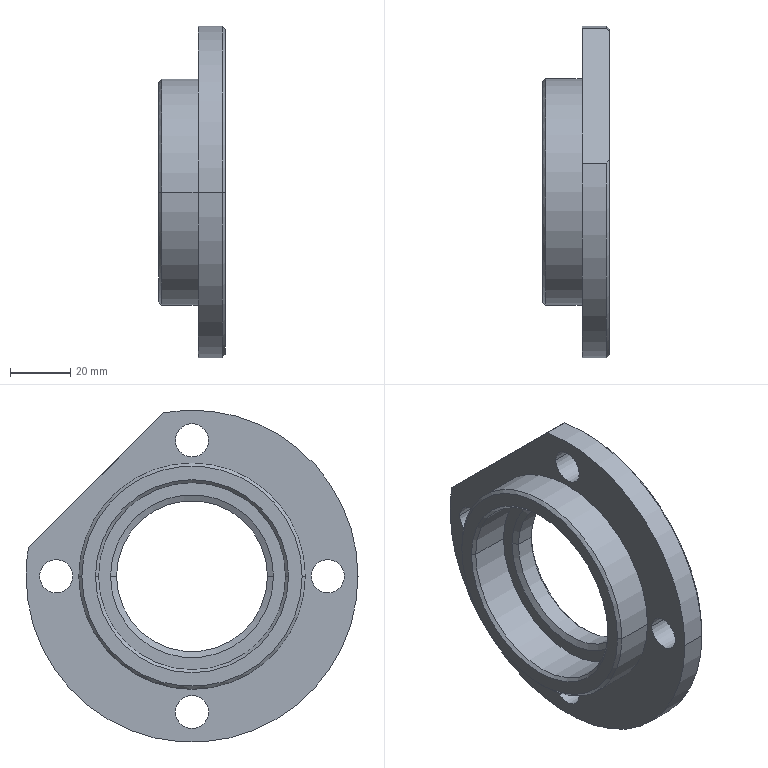Part | SolidWorks | features BaseBody 1 | 1 solid | 33 faces | box 22 x 110 x 110 mm | volume 77102 mm3 | cylinder 17 | cone 11 | plane 5 | commonest cylinder face diameters 11 x8 110 x3 50 x2 62 x2 75 x2
STEP:
#1=CARTESIAN_POINT('',(8.,-25.,0.));
#2=VERTEX_POINT('',#1);
#3=CARTESIAN_POINT('',(8.,25.,0.));
#4=VERTEX_POINT('',#3);
#5=CARTESIAN_POINT('',(8.,0.,0.));
#6=DIRECTION('',(1.,0.,0.));
#7=DIRECTION('',(0.,-1.,0.));
#8=AXIS2_PLACEMENT_3D('',#5,#6,#7);
#9=CIRCLE('',#8,25.);
#10=EDGE_CURVE('',#2,#4,#9,.T.);
#11=ORIENTED_EDGE('',*,*,#10,.F.);
#12=CARTESIAN_POINT('',(9.,-26.,0.));
#13=VERTEX_POINT('',#12);
#14=CARTESIAN_POINT('',(9.,-26.,0.));
#15=DIRECTION('',(0.7071,-0.7071,0.));
#16=VECTOR('',#15,1000.);
#17=LINE('',#14,#16);
#18=EDGE_CURVE('',#2,#13,#17,.T.);
#19=ORIENTED_EDGE('',*,*,#18,.T.);
#20=CARTESIAN_POINT('',(9.,26.,0.));
#21=VERTEX_POINT('',#20);
#22=CARTESIAN_POINT('',(9.,0.,0.));
#23=DIRECTION('',(-1.,0.,0.));
#24=DIRECTION('',(0.,1.,0.));
#25=AXIS2_PLACEMENT_3D('',#22,#23,#24);
#26=CIRCLE('',#25,26.);
#27=EDGE_CURVE('',#21,#13,#26,.T.);
#28=ORIENTED_EDGE('',*,*,#27,.F.);
#29=CARTESIAN_POINT('',(9.,26.,0.));
#30=DIRECTION('',(0.7071,0.7071,0.));
#31=VECTOR('',#30,1000.);
#32=LINE('',#29,#31);
#33=EDGE_CURVE('',#4,#21,#32,.T.);
#34=ORIENTED_EDGE('',*,*,#33,.F.);
#35=EDGE_LOOP('',(#11,#19,#28,#34));
#36=FACE_OUTER_BOUND('',#35,.T.);
#37=CARTESIAN_POINT('',(9.,0.,0.));
#38=DIRECTION('',(1.,0.,0.));
#39=DIRECTION('',(0.,1.,0.));
#40=AXIS2_PLACEMENT_3D('',#37,#38,#39);
#41=CONICAL_SURFACE('',#40,26.,0.7854);
#42=ADVANCED_FACE('',(#36),#41,.F.);
#43=CARTESIAN_POINT('',(0.,39.5,0.));
#44=VERTEX_POINT('',#43);
#45=CARTESIAN_POINT('',(0.,50.5,0.));
#46=VERTEX_POINT('',#45);
#47=CARTESIAN_POINT('',(0.,45.,0.));
#48=DIRECTION('',(1.,0.,0.));
#49=DIRECTION('',(0.,1.,0.));
#50=AXIS2_PLACEMENT_3D('',#47,#48,#49);
#51=CIRCLE('',#50,5.5);
#52=EDGE_CURVE('',#44,#46,#51,.T.);
#53=ORIENTED_EDGE('',*,*,#52,.F.);
#54=CARTESIAN_POINT('',(9.,39.5,0.));
#55=VERTEX_POINT('',#54);
#56=CARTESIAN_POINT('',(-148.111,39.5,0.));
#57=DIRECTION('',(1.,0.,0.));
#58=VECTOR('',#57,1000.);
#59=LINE('',#56,#58);
#60=EDGE_CURVE('',#44,#55,#59,.T.);
#61=ORIENTED_EDGE('',*,*,#60,.T.);
#62=CARTESIAN_POINT('',(9.,50.5,0.));
#63=VERTEX_POINT('',#62);
#64=CARTESIAN_POINT('',(9.,45.,0.));
#65=DIRECTION('',(-1.,0.,0.));
#66=DIRECTION('',(0.,1.,0.));
#67=AXIS2_PLACEMENT_3D('',#64,#65,#66);
#68=CIRCLE('',#67,5.5);
#69=EDGE_CURVE('',#63,#55,#68,.T.);
#70=ORIENTED_EDGE('',*,*,#69,.F.);
#71=CARTESIAN_POINT('',(-148.111,50.5,0.));
#72=DIRECTION('',(1.,0.,0.));
#73=VECTOR('',#72,1000.);
#74=LINE('',#71,#73);
#75=EDGE_CURVE('',#46,#63,#74,.T.);
#76=ORIENTED_EDGE('',*,*,#75,.F.);
#77=EDGE_LOOP('',(#53,#61,#70,#76));
#78=FACE_OUTER_BOUND('',#77,.T.);
#79=CARTESIAN_POINT('',(-148.111,45.,0.));
#80=DIRECTION('',(1.,0.,0.));
#81=DIRECTION('',(0.,1.,0.));
#82=AXIS2_PLACEMENT_3D('',#79,#80,#81);
#83=CYLINDRICAL_SURFACE('',#82,5.5);
#84=ADVANCED_FACE('',(#78),#83,.F.);
#85=CARTESIAN_POINT('',(0.,-5.5,45.));
#86=VERTEX_POINT('',#85);
#87=CARTESIAN_POINT('',(0.,5.5,45.));
#88=VERTEX_POINT('',#87);
#89=CARTESIAN_POINT('',(0.,0.,45.));
#90=DIRECTION('',(1.,0.,0.));
#91=DIRECTION('',(0.,1.,0.));
#92=AXIS2_PLACEMENT_3D('',#89,#90,#91);
#93=CIRCLE('',#92,5.5);
#94=EDGE_CURVE('',#86,#88,#93,.T.);
#95=ORIENTED_EDGE('',*,*,#94,.F.);
#96=CARTESIAN_POINT('',(9.,-5.5,45.));
#97=VERTEX_POINT('',#96);
#98=CARTESIAN_POINT('',(-148.111,-5.5,45.));
#99=DIRECTION('',(1.,0.,0.));
#100=VECTOR('',#99,1000.);
#101=LINE('',#98,#100);
#102=EDGE_CURVE('',#86,#97,#101,.T.);
#103=ORIENTED_EDGE('',*,*,#102,.T.);
#104=CARTESIAN_POINT('',(9.,5.5,45.));
#105=VERTEX_POINT('',#104);
#106=CARTESIAN_POINT('',(9.,0.,45.));
#107=DIRECTION('',(-1.,0.,0.));
#108=DIRECTION('',(0.,1.,0.));
#109=AXIS2_PLACEMENT_3D('',#106,#107,#108);
#110=CIRCLE('',#109,5.5);
#111=EDGE_CURVE('',#105,#97,#110,.T.);
#112=ORIENTED_EDGE('',*,*,#111,.F.);
#113=CARTESIAN_POINT('',(-148.111,5.5,45.));
#114=DIRECTION('',(1.,0.,0.));
#115=VECTOR('',#114,1000.);
#116=LINE('',#113,#115);
#117=EDGE_CURVE('',#88,#105,#116,.T.);
#118=ORIENTED_EDGE('',*,*,#117,.F.);
#119=EDGE_LOOP('',(#95,#103,#112,#118));
#120=FACE_OUTER_BOUND('',#119,.T.);
#121=CARTESIAN_POINT('',(-148.111,0.,45.));
#122=DIRECTION('',(1.,0.,0.));
#123=DIRECTION('',(0.,1.,0.));
#124=AXIS2_PLACEMENT_3D('',#121,#122,#123);
#125=CYLINDRICAL_SURFACE('',#124,5.5);
#126=ADVANCED_FACE('',(#120),#125,.F.);
#127=CARTESIAN_POINT('',(0.,-50.5,0.));
#128=VERTEX_POINT('',#127);
#129=CARTESIAN_POINT('',(0.,-39.5,0.));
#130=VERTEX_POINT('',#129);
#131=CARTESIAN_POINT('',(0.,-45.,0.));
#132=DIRECTION('',(1.,0.,0.));
#133=DIRECTION('',(0.,1.,0.));
#134=AXIS2_PLACEMENT_3D('',#131,#132,#133);
#135=CIRCLE('',#134,5.5);
#136=EDGE_CURVE('',#128,#130,#135,.T.);
#137=ORIENTED_EDGE('',*,*,#136,.F.);
#138=CARTESIAN_POINT('',(9.,-50.5,0.));
#139=VERTEX_POINT('',#138);
#140=CARTESIAN_POINT('',(-148.111,-50.5,0.));
#141=DIRECTION('',(1.,0.,0.));
#142=VECTOR('',#141,1000.);
#143=LINE('',#140,#142);
#144=EDGE_CURVE('',#128,#139,#143,.T.);
#145=ORIENTED_EDGE('',*,*,#144,.T.);
#146=CARTESIAN_POINT('',(9.,-39.5,0.));
#147=VERTEX_POINT('',#146);
#148=CARTESIAN_POINT('',(9.,-45.,0.));
#149=DIRECTION('',(-1.,0.,0.));
#150=DIRECTION('',(0.,1.,0.));
#151=AXIS2_PLACEMENT_3D('',#148,#149,#150);
#152=CIRCLE('',#151,5.5);
#153=EDGE_CURVE('',#147,#139,#152,.T.);
#154=ORIENTED_EDGE('',*,*,#153,.F.);
#155=CARTESIAN_POINT('',(-148.111,-39.5,0.));
#156=DIRECTION('',(1.,0.,0.));
#157=VECTOR('',#156,1000.);
#158=LINE('',#155,#157);
#159=EDGE_CURVE('',#130,#147,#158,.T.);
#160=ORIENTED_EDGE('',*,*,#159,.F.);
#161=EDGE_LOOP('',(#137,#145,#154,#160));
#162=FACE_OUTER_BOUND('',#161,.T.);
#163=CARTESIAN_POINT('',(-148.111,-45.,0.));
#164=DIRECTION('',(1.,0.,0.));
#165=DIRECTION('',(0.,1.,0.));
#166=AXIS2_PLACEMENT_3D('',#163,#164,#165);
#167=CYLINDRICAL_SURFACE('',#166,5.5);
#168=ADVANCED_FACE('',(#162),#167,.F.);
#169=CARTESIAN_POINT('',(0.,-5.5,-45.));
#170=VERTEX_POINT('',#169);
#171=CARTESIAN_POINT('',(0.,5.5,-45.));
#172=VERTEX_POINT('',#171);
#173=CARTESIAN_POINT('',(0.,0.,-45.));
#174=DIRECTION('',(1.,0.,0.));
#175=DIRECTION('',(0.,1.,0.));
#176=AXIS2_PLACEMENT_3D('',#173,#174,#175);
#177=CIRCLE('',#176,5.5);
#178=EDGE_CURVE('',#170,#172,#177,.T.);
#179=ORIENTED_EDGE('',*,*,#178,.F.);
#180=CARTESIAN_POINT('',(9.,-5.5,-45.));
#181=VERTEX_POINT('',#180);
#182=CARTESIAN_POINT('',(-148.111,-5.5,-45.));
#183=DIRECTION('',(1.,0.,0.));
#184=VECTOR('',#183,1000.);
#185=LINE('',#182,#184);
#186=EDGE_CURVE('',#170,#181,#185,.T.);
#187=ORIENTED_EDGE('',*,*,#186,.T.);
#188=CARTESIAN_POINT('',(9.,5.5,-45.));
#189=VERTEX_POINT('',#188);
#190=CARTESIAN_POINT('',(9.,0.,-45.));
#191=DIRECTION('',(-1.,0.,0.));
#192=DIRECTION('',(0.,1.,0.));
#193=AXIS2_PLACEMENT_3D('',#190,#191,#192);
#194=CIRCLE('',#193,5.5);
#195=EDGE_CURVE('',#189,#181,#194,.T.);
#196=ORIENTED_EDGE('',*,*,#195,.F.);
#197=CARTESIAN_POINT('',(-148.111,5.5,-45.));
#198=DIRECTION('',(1.,0.,0.));
#199=VECTOR('',#198,1000.);
#200=LINE('',#197,#199);
#201=EDGE_CURVE('',#172,#189,#200,.T.);
#202=ORIENTED_EDGE('',*,*,#201,.F.);
#203=EDGE_LOOP('',(#179,#187,#196,#202));
#204=FACE_OUTER_BOUND('',#203,.T.);
#205=CARTESIAN_POINT('',(-148.111,0.,-45.));
#206=DIRECTION('',(1.,0.,0.));
#207=DIRECTION('',(0.,1.,0.));
#208=AXIS2_PLACEMENT_3D('',#205,#206,#207);
#209=CYLINDRICAL_SURFACE('',#208,5.5);
#210=ADVANCED_FACE('',(#204),#209,.F.);
#211=CARTESIAN_POINT('',(9.,54.,0.));
#212=VERTEX_POINT('',#211);
#213=CARTESIAN_POINT('',(9.,52.927,10.713));
#214=VERTEX_POINT('',#213);
#215=CARTESIAN_POINT('',(9.,0.,0.));
#216=DIRECTION('',(1.,0.,0.));
#217=DIRECTION('',(0.,-1.,0.));
#218=AXIS2_PLACEMENT_3D('',#215,#216,#217);
#219=CIRCLE('',#218,54.);
#220=EDGE_CURVE('',#212,#214,#219,.T.);
#221=ORIENTED_EDGE('',*,*,#220,.F.);
#222=CARTESIAN_POINT('',(8.,55.,0.));
#223=VERTEX_POINT('',#222);
#224=CARTESIAN_POINT('',(8.,55.,0.));
#225=DIRECTION('',(-0.7071,0.7071,0.));
#226=VECTOR('',#225,1000.);
#227=LINE('',#224,#226);
#228=EDGE_CURVE('',#212,#223,#227,.T.);
#229=ORIENTED_EDGE('',*,*,#228,.T.);
#230=CARTESIAN_POINT('',(8.,54.18,9.459));
#231=VERTEX_POINT('',#230);
#232=CARTESIAN_POINT('',(8.,0.,0.));
#233=DIRECTION('',(1.,0.,0.));
#234=DIRECTION('',(0.,-1.,0.));
#235=AXIS2_PLACEMENT_3D('',#232,#233,#234);
#236=CIRCLE('',#235,55.);
#237=EDGE_CURVE('',#223,#231,#236,.T.);
#238=ORIENTED_EDGE('',*,*,#237,.T.);
#239=CARTESIAN_POINT('',(8.,54.18,9.459));
#240=CARTESIAN_POINT('',(8.338,53.765,9.875));
#241=CARTESIAN_POINT('',(8.672,53.347,10.293));
#242=CARTESIAN_POINT('',(9.,52.927,10.713));
#243=B_SPLINE_CURVE_WITH_KNOTS('',3,(#239,#240,#241,#242),.UNSPECIFIED.,.F.,.F.,(4,4),(0.,0.002036),.UNSPECIFIED.);
#244=EDGE_CURVE('',#231,#214,#243,.T.);
#245=ORIENTED_EDGE('',*,*,#244,.T.);
#246=EDGE_LOOP('',(#221,#229,#238,#245));
#247=FACE_OUTER_BOUND('',#246,.T.);
#248=CARTESIAN_POINT('',(8.,0.,0.));
#249=DIRECTION('',(-1.,0.,0.));
#250=DIRECTION('',(0.,-1.,0.));
#251=AXIS2_PLACEMENT_3D('',#248,#249,#250);
#252=CONICAL_SURFACE('',#251,55.,0.7854);
#253=ADVANCED_FACE('',(#247),#252,.T.);
#254=ORIENTED_EDGE('',*,*,#228,.F.);
#255=CARTESIAN_POINT('',(9.,-54.,0.));
#256=VERTEX_POINT('',#255);
#257=CARTESIAN_POINT('',(9.,0.,0.));
#258=DIRECTION('',(1.,0.,0.));
#259=DIRECTION('',(0.,-1.,0.));
#260=AXIS2_PLACEMENT_3D('',#257,#258,#259);
#261=CIRCLE('',#260,54.);
#262=EDGE_CURVE('',#256,#212,#261,.T.);
#263=ORIENTED_EDGE('',*,*,#262,.F.);
#264=CARTESIAN_POINT('',(8.,-55.,0.));
#265=VERTEX_POINT('',#264);
#266=CARTESIAN_POINT('',(8.,-55.,0.));
#267=DIRECTION('',(-0.7071,-0.7071,0.));
#268=VECTOR('',#267,1000.);
#269=LINE('',#266,#268);
#270=EDGE_CURVE('',#256,#265,#269,.T.);
#271=ORIENTED_EDGE('',*,*,#270,.T.);
#272=CARTESIAN_POINT('',(8.,0.,0.));
#273=DIRECTION('',(1.,0.,0.));
#274=DIRECTION('',(0.,-1.,0.));
#275=AXIS2_PLACEMENT_3D('',#272,#273,#274);
#276=CIRCLE('',#275,55.);
#277=EDGE_CURVE('',#265,#223,#276,.T.);
#278=ORIENTED_EDGE('',*,*,#277,.T.);
#279=EDGE_LOOP('',(#254,#263,#271,#278));
#280=FACE_OUTER_BOUND('',#279,.T.);
#281=CARTESIAN_POINT('',(8.,0.,0.));
#282=DIRECTION('',(-1.,0.,0.));
#283=DIRECTION('',(0.,-1.,0.));
#284=AXIS2_PLACEMENT_3D('',#281,#282,#283);
#285=CONICAL_SURFACE('',#284,55.,0.7854);
#286=ADVANCED_FACE('',(#280),#285,.T.);
#287=CARTESIAN_POINT('',(2.,-25.,0.));
#288=VERTEX_POINT('',#287);
#289=CARTESIAN_POINT('',(2.,25.,0.));
#290=VERTEX_POINT('',#289);
#291=CARTESIAN_POINT('',(2.,0.,0.));
#292=DIRECTION('',(1.,0.,0.));
#293=DIRECTION('',(0.,1.,0.));
#294=AXIS2_PLACEMENT_3D('',#291,#292,#293);
#295=CIRCLE('',#294,25.);
#296=EDGE_CURVE('',#288,#290,#295,.T.);
#297=ORIENTED_EDGE('',*,*,#296,.F.);
#298=CARTESIAN_POINT('',(5.,-25.,0.));
#299=DIRECTION('',(1.,0.,0.));
#300=VECTOR('',#299,1000.);
#301=LINE('',#298,#300);
#302=EDGE_CURVE('',#288,#2,#301,.T.);
#303=ORIENTED_EDGE('',*,*,#302,.T.);
#304=ORIENTED_EDGE('',*,*,#10,.T.);
#305=CARTESIAN_POINT('',(5.,25.,0.));
#306=DIRECTION('',(1.,0.,0.));
#307=VECTOR('',#306,1000.);
#308=LINE('',#305,#307);
#309=EDGE_CURVE('',#290,#4,#308,.T.);
#310=ORIENTED_EDGE('',*,*,#309,.F.);
#311=EDGE_LOOP('',(#297,#303,#304,#310));
#312=FACE_OUTER_BOUND('',#311,.T.);
#313=CARTESIAN_POINT('',(5.,0.,0.));
#314=DIRECTION('',(1.,0.,0.));
#315=DIRECTION('',(0.,1.,0.));
#316=AXIS2_PLACEMENT_3D('',#313,#314,#315);
#317=CYLINDRICAL_SURFACE('',#316,25.);
#318=ADVANCED_FACE('',(#312),#317,.F.);
#319=CARTESIAN_POINT('',(0.,-55.,0.));
#320=VERTEX_POINT('',#319);
#321=CARTESIAN_POINT('',(0.,9.459,54.18));
#322=VERTEX_POINT('',#321);
#323=CARTESIAN_POINT('',(0.,0.,0.));
#324=DIRECTION('',(-1.,0.,0.));
#325=DIRECTION('',(0.,1.,0.));
#326=AXIS2_PLACEMENT_3D('',#323,#324,#325);
#327=CIRCLE('',#326,55.);
#328=EDGE_CURVE('',#320,#322,#327,.T.);
#329=ORIENTED_EDGE('',*,*,#328,.F.);
#330=CARTESIAN_POINT('',(4.5,-55.,0.));
#331=DIRECTION('',(1.,0.,0.));
#332=VECTOR('',#331,1000.);
#333=LINE('',#330,#332);
#334=EDGE_CURVE('',#320,#265,#333,.T.);
#335=ORIENTED_EDGE('',*,*,#334,.T.);
#336=CARTESIAN_POINT('',(8.,9.459,54.18));
#337=VERTEX_POINT('',#336);
#338=CARTESIAN_POINT('',(8.,0.,0.));
#339=DIRECTION('',(1.,0.,0.));
#340=DIRECTION('',(0.,-1.,0.));
#341=AXIS2_PLACEMENT_3D('',#338,#339,#340);
#342=CIRCLE('',#341,55.);
#343=EDGE_CURVE('',#337,#265,#342,.T.);
#344=ORIENTED_EDGE('',*,*,#343,.F.);
#345=CARTESIAN_POINT('',(9.,9.459,54.18));
#346=DIRECTION('',(-1.,0.,0.));
#347=VECTOR('',#346,1000.);
#348=LINE('',#345,#347);
#349=EDGE_CURVE('',#337,#322,#348,.T.);
#350=ORIENTED_EDGE('',*,*,#349,.T.);
#351=EDGE_LOOP('',(#329,#335,#344,#350));
#352=FACE_OUTER_BOUND('',#351,.T.);
#353=CARTESIAN_POINT('',(4.5,0.,0.));
#354=DIRECTION('',(1.,0.,0.));
#355=DIRECTION('',(0.,1.,0.));
#356=AXIS2_PLACEMENT_3D('',#353,#354,#355);
#357=CYLINDRICAL_SURFACE('',#356,55.);
#358=ADVANCED_FACE('',(#352),#357,.T.);
#359=ORIENTED_EDGE('',*,*,#334,.F.);
#360=CARTESIAN_POINT('',(0.,55.,0.));
#361=VERTEX_POINT('',#360);
#362=CARTESIAN_POINT('',(0.,0.,0.));
#363=DIRECTION('',(-1.,0.,0.));
#364=DIRECTION('',(0.,1.,0.));
#365=AXIS2_PLACEMENT_3D('',#362,#363,#364);
#366=CIRCLE('',#365,55.);
#367=EDGE_CURVE('',#361,#320,#366,.T.);
#368=ORIENTED_EDGE('',*,*,#367,.F.);
#369=CARTESIAN_POINT('',(4.5,55.,0.));
#370=DIRECTION('',(1.,0.,0.));
#371=VECTOR('',#370,1000.);
#372=LINE('',#369,#371);
#373=EDGE_CURVE('',#361,#223,#372,.T.);
#374=ORIENTED_EDGE('',*,*,#373,.T.);
#375=ORIENTED_EDGE('',*,*,#277,.F.);
#376=EDGE_LOOP('',(#359,#368,#374,#375));
#377=FACE_OUTER_BOUND('',#376,.T.);
#378=CARTESIAN_POINT('',(4.5,0.,0.));
#379=DIRECTION('',(1.,0.,0.));
#380=DIRECTION('',(0.,1.,0.));
#381=AXIS2_PLACEMENT_3D('',#378,#379,#380);
#382=CYLINDRICAL_SURFACE('',#381,55.);
#383=ADVANCED_FACE('',(#377),#382,.T.);
#384=ORIENTED_EDGE('',*,*,#296,.T.);
#385=CARTESIAN_POINT('',(1.,27.,0.));
#386=VERTEX_POINT('',#385);
#387=CARTESIAN_POINT('',(1.,27.,0.));
#388=DIRECTION('',(-0.4472,0.8944,0.));
#389=VECTOR('',#388,1000.);
#390=LINE('',#387,#389);
#391=EDGE_CURVE('',#290,#386,#390,.T.);
#392=ORIENTED_EDGE('',*,*,#391,.T.);
#393=CARTESIAN_POINT('',(1.,-27.,0.));
#394=VERTEX_POINT('',#393);
#395=CARTESIAN_POINT('',(1.,0.,0.));
#396=DIRECTION('',(1.,0.,0.));
#397=DIRECTION('',(0.,-1.,0.));
#398=AXIS2_PLACEMENT_3D('',#395,#396,#397);
#399=CIRCLE('',#398,27.);
#400=EDGE_CURVE('',#394,#386,#399,.T.);
#401=ORIENTED_EDGE('',*,*,#400,.F.);
#402=CARTESIAN_POINT('',(1.,-27.,0.));
#403=DIRECTION('',(-0.4472,-0.8944,0.));
#404=VECTOR('',#403,1000.);
#405=LINE('',#402,#404);
#406=EDGE_CURVE('',#288,#394,#405,.T.);
#407=ORIENTED_EDGE('',*,*,#406,.F.);
#408=EDGE_LOOP('',(#384,#392,#401,#407));
#409=FACE_OUTER_BOUND('',#408,.T.);
#410=CARTESIAN_POINT('',(1.,0.,0.));
#411=DIRECTION('',(-1.,0.,0.));
#412=DIRECTION('',(0.,-1.,0.));
#413=AXIS2_PLACEMENT_3D('',#410,#411,#412);
#414=CONICAL_SURFACE('',#413,27.,1.107);
#415=ADVANCED_FACE('',(#409),#414,.F.);
#416=CARTESIAN_POINT('',(-12.,37.5,0.));
#417=VERTEX_POINT('',#416);
#418=CARTESIAN_POINT('',(-12.,-37.5,0.));
#419=VERTEX_POINT('',#418);
#420=CARTESIAN_POINT('',(-12.,0.,0.));
#421=DIRECTION('',(1.,0.,0.));
#422=DIRECTION('',(0.,1.,0.));
#423=AXIS2_PLACEMENT_3D('',#420,#421,#422);
#424=CIRCLE('',#423,37.5);
#425=EDGE_CURVE('',#417,#419,#424,.T.);
#426=ORIENTED_EDGE('',*,*,#425,.T.);
#427=CARTESIAN_POINT('',(0.,-37.5,0.));
#428=VERTEX_POINT('',#427);
#429=CARTESIAN_POINT('',(-6.5,-37.5,0.));
#430=DIRECTION('',(1.,0.,0.));
#431=VECTOR('',#430,1000.);
#432=LINE('',#429,#431);
#433=EDGE_CURVE('',#419,#428,#432,.T.);
#434=ORIENTED_EDGE('',*,*,#433,.T.);
#435=CARTESIAN_POINT('',(0.,37.5,0.));
#436=VERTEX_POINT('',#435);
#437=CARTESIAN_POINT('',(0.,0.,0.));
#438=DIRECTION('',(1.,0.,0.));
#439=DIRECTION('',(0.,1.,0.));
#440=AXIS2_PLACEMENT_3D('',#437,#438,#439);
#441=CIRCLE('',#440,37.5);
#442=EDGE_CURVE('',#436,#428,#441,.T.);
#443=ORIENTED_EDGE('',*,*,#442,.F.);
#444=CARTESIAN_POINT('',(-6.5,37.5,0.));
#445=DIRECTION('',(1.,0.,0.));
#446=VECTOR('',#445,1000.);
#447=LINE('',#444,#446);
#448=EDGE_CURVE('',#417,#436,#447,.T.);
#449=ORIENTED_EDGE('',*,*,#448,.F.);
#450=EDGE_LOOP('',(#426,#434,#443,#449));
#451=FACE_OUTER_BOUND('',#450,.T.);
#452=CARTESIAN_POINT('',(-6.5,0.,0.));
#453=DIRECTION('',(1.,0.,0.));
#454=DIRECTION('',(0.,1.,0.));
#455=AXIS2_PLACEMENT_3D('',#452,#453,#454);
#456=CYLINDRICAL_SURFACE('',#455,37.5);
#457=ADVANCED_FACE('',(#451),#456,.T.);
#458=CARTESIAN_POINT('',(-13.,36.5,0.));
#459=VERTEX_POINT('',#458);
#460=CARTESIAN_POINT('',(-13.,-36.5,0.));
#461=VERTEX_POINT('',#460);
#462=CARTESIAN_POINT('',(-13.,0.,0.));
#463=DIRECTION('',(1.,0.,0.));
#464=DIRECTION('',(0.,1.,0.));
#465=AXIS2_PLACEMENT_3D('',#462,#463,#464);
#466=CIRCLE('',#465,36.5);
#467=EDGE_CURVE('',#459,#461,#466,.T.);
#468=ORIENTED_EDGE('',*,*,#467,.T.);
#469=CARTESIAN_POINT('',(-12.,-37.5,0.));
#470=DIRECTION('',(0.7071,-0.7071,0.));
#471=VECTOR('',#470,1000.);
#472=LINE('',#469,#471);
#473=EDGE_CURVE('',#461,#419,#472,.T.);
#474=ORIENTED_EDGE('',*,*,#473,.T.);
#475=ORIENTED_EDGE('',*,*,#425,.F.);
#476=CARTESIAN_POINT('',(-12.,37.5,0.));
#477=DIRECTION('',(0.7071,0.7071,0.));
#478=VECTOR('',#477,1000.);
#479=LINE('',#476,#478);
#480=EDGE_CURVE('',#459,#417,#479,.T.);
#481=ORIENTED_EDGE('',*,*,#480,.F.);
#482=EDGE_LOOP('',(#468,#474,#475,#481));
#483=FACE_OUTER_BOUND('',#482,.T.);
#484=CARTESIAN_POINT('',(-12.,0.,0.));
#485=DIRECTION('',(1.,0.,0.));
#486=DIRECTION('',(0.,1.,0.));
#487=AXIS2_PLACEMENT_3D('',#484,#485,#486);
#488=CONICAL_SURFACE('',#487,37.5,0.7854);
#489=ADVANCED_FACE('',(#483),#488,.T.);
#490=CARTESIAN_POINT('',(-12.,-31.,0.));
#491=VERTEX_POINT('',#490);
#492=CARTESIAN_POINT('',(-12.,31.,0.));
#493=VERTEX_POINT('',#492);
#494=CARTESIAN_POINT('',(-12.,0.,0.));
#495=DIRECTION('',(1.,0.,0.));
#496=DIRECTION('',(0.,1.,0.));
#497=AXIS2_PLACEMENT_3D('',#494,#495,#496);
#498=CIRCLE('',#497,31.);
#499=EDGE_CURVE('',#491,#493,#498,.T.);
#500=ORIENTED_EDGE('',*,*,#499,.F.);
#501=CARTESIAN_POINT('',(1.,-31.,0.));
#502=VERTEX_POINT('',#501);
#503=CARTESIAN_POINT('',(-6.,-31.,0.));
#504=DIRECTION('',(1.,0.,0.));
#505=VECTOR('',#504,1000.);
#506=LINE('',#503,#505);
#507=EDGE_CURVE('',#491,#502,#506,.T.);
#508=ORIENTED_EDGE('',*,*,#507,.T.);
#509=CARTESIAN_POINT('',(1.,31.,0.));
#510=VERTEX_POINT('',#509);
#511=CARTESIAN_POINT('',(1.,0.,0.));
#512=DIRECTION('',(-1.,0.,0.));
#513=DIRECTION('',(0.,1.,0.));
#514=AXIS2_PLACEMENT_3D('',#511,#512,#513);
#515=CIRCLE('',#514,31.);
#516=EDGE_CURVE('',#510,#502,#515,.T.);
#517=ORIENTED_EDGE('',*,*,#516,.F.);
#518=CARTESIAN_POINT('',(-6.,31.,0.));
#519=DIRECTION('',(1.,0.,0.));
#520=VECTOR('',#519,1000.);
#521=LINE('',#518,#520);
#522=EDGE_CURVE('',#493,#510,#521,.T.);
#523=ORIENTED_EDGE('',*,*,#522,.F.);
#524=EDGE_LOOP('',(#500,#508,#517,#523));
#525=FACE_OUTER_BOUND('',#524,.T.);
#526=CARTESIAN_POINT('',(-6.,0.,0.));
#527=DIRECTION('',(1.,0.,0.));
#528=DIRECTION('',(0.,1.,0.));
#529=AXIS2_PLACEMENT_3D('',#526,#527,#528);
#530=CYLINDRICAL_SURFACE('',#529,31.);
#531=ADVANCED_FACE('',(#525),#530,.F.);
#532=ORIENTED_EDGE('',*,*,#499,.T.);
#533=CARTESIAN_POINT('',(-13.,32.,0.));
#534=VERTEX_POINT('',#533);
#535=CARTESIAN_POINT('',(-13.,32.,0.));
#536=DIRECTION('',(-0.7071,0.7071,0.));
#537=VECTOR('',#536,1000.);
#538=LINE('',#535,#537);
#539=EDGE_CURVE('',#493,#534,#538,.T.);
#540=ORIENTED_EDGE('',*,*,#539,.T.);
#541=CARTESIAN_POINT('',(-13.,-32.,0.));
#542=VERTEX_POINT('',#541);
#543=CARTESIAN_POINT('',(-13.,0.,0.));
#544=DIRECTION('',(1.,0.,0.));
#545=DIRECTION('',(0.,-1.,0.));
#546=AXIS2_PLACEMENT_3D('',#543,#544,#545);
#547=CIRCLE('',#546,32.);
#548=EDGE_CURVE('',#542,#534,#547,.T.);
#549=ORIENTED_EDGE('',*,*,#548,.F.);
#550=CARTESIAN_POINT('',(-13.,-32.,0.));
#551=DIRECTION('',(-0.7071,-0.7071,0.));
#552=VECTOR('',#551,1000.);
#553=LINE('',#550,#552);
#554=EDGE_CURVE('',#491,#542,#553,.T.);
#555=ORIENTED_EDGE('',*,*,#554,.F.);
#556=EDGE_LOOP('',(#532,#540,#549,#555));
#557=FACE_OUTER_BOUND('',#556,.T.);
#558=CARTESIAN_POINT('',(-13.,0.,0.));
#559=DIRECTION('',(-1.,0.,0.));
#560=DIRECTION('',(0.,-1.,0.));
#561=AXIS2_PLACEMENT_3D('',#558,#559,#560);
#562=CONICAL_SURFACE('',#561,32.,0.7854);
#563=ADVANCED_FACE('',(#557),#562,.F.);
#564=ORIENTED_EDGE('',*,*,#27,.T.);
#565=CARTESIAN_POINT('',(9.,0.,0.));
#566=DIRECTION('',(-1.,0.,0.));
#567=DIRECTION('',(0.,1.,0.));
#568=AXIS2_PLACEMENT_3D('',#565,#566,#567);
#569=CIRCLE('',#568,26.);
#570=EDGE_CURVE('',#13,#21,#569,.T.);
#571=ORIENTED_EDGE('',*,*,#570,.T.);
#572=EDGE_LOOP('',(#564,#571));
#573=FACE_BOUND('',#572,.T.);
#574=ORIENTED_EDGE('',*,*,#69,.T.);
#575=CARTESIAN_POINT('',(9.,45.,0.));
#576=DIRECTION('',(-1.,0.,0.));
#577=DIRECTION('',(0.,1.,0.));
#578=AXIS2_PLACEMENT_3D('',#575,#576,#577);
#579=CIRCLE('',#578,5.5);
#580=EDGE_CURVE('',#55,#63,#579,.T.);
#581=ORIENTED_EDGE('',*,*,#580,.T.);
#582=EDGE_LOOP('',(#574,#581));
#583=FACE_BOUND('',#582,.T.);
#584=ORIENTED_EDGE('',*,*,#111,.T.);
#585=CARTESIAN_POINT('',(9.,0.,45.));
#586=DIRECTION('',(-1.,0.,0.));
#587=DIRECTION('',(0.,1.,0.));
#588=AXIS2_PLACEMENT_3D('',#585,#586,#587);
#589=CIRCLE('',#588,5.5);
#590=EDGE_CURVE('',#97,#105,#589,.T.);
#591=ORIENTED_EDGE('',*,*,#590,.T.);
#592=EDGE_LOOP('',(#584,#591));
#593=FACE_BOUND('',#592,.T.);
#594=ORIENTED_EDGE('',*,*,#153,.T.);
#595=CARTESIAN_POINT('',(9.,-45.,0.));
#596=DIRECTION('',(-1.,0.,0.));
#597=DIRECTION('',(0.,1.,0.));
#598=AXIS2_PLACEMENT_3D('',#595,#596,#597);
#599=CIRCLE('',#598,5.5);
#600=EDGE_CURVE('',#139,#147,#599,.T.);
#601=ORIENTED_EDGE('',*,*,#600,.T.);
#602=EDGE_LOOP('',(#594,#601));
#603=FACE_BOUND('',#602,.T.);
#604=ORIENTED_EDGE('',*,*,#195,.T.);
#605=CARTESIAN_POINT('',(9.,0.,-45.));
#606=DIRECTION('',(-1.,0.,0.));
#607=DIRECTION('',(0.,1.,0.));
#608=AXIS2_PLACEMENT_3D('',#605,#606,#607);
#609=CIRCLE('',#608,5.5);
#610=EDGE_CURVE('',#181,#189,#609,.T.);
#611=ORIENTED_EDGE('',*,*,#610,.T.);
#612=EDGE_LOOP('',(#604,#611));
#613=FACE_BOUND('',#612,.T.);
#614=CARTESIAN_POINT('',(9.,10.713,52.927));
#615=VERTEX_POINT('',#614);
#616=CARTESIAN_POINT('',(9.,52.927,10.713));
#617=DIRECTION('',(0.,-0.7071,0.7071));
#618=VECTOR('',#617,1000.);
#619=LINE('',#616,#618);
#620=EDGE_CURVE('',#214,#615,#619,.T.);
#621=ORIENTED_EDGE('',*,*,#620,.T.);
#622=CARTESIAN_POINT('',(9.,0.,0.));
#623=DIRECTION('',(1.,0.,0.));
#624=DIRECTION('',(0.,-1.,0.));
#625=AXIS2_PLACEMENT_3D('',#622,#623,#624);
#626=CIRCLE('',#625,54.);
#627=EDGE_CURVE('',#615,#256,#626,.T.);
#628=ORIENTED_EDGE('',*,*,#627,.T.);
#629=ORIENTED_EDGE('',*,*,#262,.T.);
#630=ORIENTED_EDGE('',*,*,#220,.T.);
#631=EDGE_LOOP('',(#621,#628,#629,#630));
#632=FACE_OUTER_BOUND('',#631,.T.);
#633=CARTESIAN_POINT('',(9.,25.,0.));
#634=DIRECTION('',(1.,0.,0.));
#635=DIRECTION('',(0.,1.,0.));
#636=AXIS2_PLACEMENT_3D('',#633,#634,#635);
#637=PLANE('',#636);
#638=ADVANCED_FACE('',(#573,#583,#593,#603,#613,#632),#637,.T.);
#639=ORIENTED_EDGE('',*,*,#18,.F.);
#640=CARTESIAN_POINT('',(8.,0.,0.));
#641=DIRECTION('',(1.,0.,0.));
#642=DIRECTION('',(0.,-1.,0.));
#643=AXIS2_PLACEMENT_3D('',#640,#641,#642);
#644=CIRCLE('',#643,25.);
#645=EDGE_CURVE('',#4,#2,#644,.T.);
#646=ORIENTED_EDGE('',*,*,#645,.F.);
#647=ORIENTED_EDGE('',*,*,#33,.T.);
#648=ORIENTED_EDGE('',*,*,#570,.F.);
#649=EDGE_LOOP('',(#639,#646,#647,#648));
#650=FACE_OUTER_BOUND('',#649,.T.);
#651=CARTESIAN_POINT('',(9.,0.,0.));
#652=DIRECTION('',(1.,0.,0.));
#653=DIRECTION('',(0.,1.,0.));
#654=AXIS2_PLACEMENT_3D('',#651,#652,#653);
#655=CONICAL_SURFACE('',#654,26.,0.7854);
#656=ADVANCED_FACE('',(#650),#655,.F.);
#657=ORIENTED_EDGE('',*,*,#60,.F.);
#658=CARTESIAN_POINT('',(0.,45.,0.));
#659=DIRECTION('',(1.,0.,0.));
#660=DIRECTION('',(0.,1.,0.));
#661=AXIS2_PLACEMENT_3D('',#658,#659,#660);
#662=CIRCLE('',#661,5.5);
#663=EDGE_CURVE('',#46,#44,#662,.T.);
#664=ORIENTED_EDGE('',*,*,#663,.F.);
#665=ORIENTED_EDGE('',*,*,#75,.T.);
#666=ORIENTED_EDGE('',*,*,#580,.F.);
#667=EDGE_LOOP('',(#657,#664,#665,#666));
#668=FACE_OUTER_BOUND('',#667,.T.);
#669=CARTESIAN_POINT('',(-148.111,45.,0.));
#670=DIRECTION('',(1.,0.,0.));
#671=DIRECTION('',(0.,1.,0.));
#672=AXIS2_PLACEMENT_3D('',#669,#670,#671);
#673=CYLINDRICAL_SURFACE('',#672,5.5);
#674=ADVANCED_FACE('',(#668),#673,.F.);
#675=ORIENTED_EDGE('',*,*,#102,.F.);
#676=CARTESIAN_POINT('',(0.,0.,45.));
#677=DIRECTION('',(1.,0.,0.));
#678=DIRECTION('',(0.,1.,0.));
#679=AXIS2_PLACEMENT_3D('',#676,#677,#678);
#680=CIRCLE('',#679,5.5);
#681=EDGE_CURVE('',#88,#86,#680,.T.);
#682=ORIENTED_EDGE('',*,*,#681,.F.);
#683=ORIENTED_EDGE('',*,*,#117,.T.);
#684=ORIENTED_EDGE('',*,*,#590,.F.);
#685=EDGE_LOOP('',(#675,#682,#683,#684));
#686=FACE_OUTER_BOUND('',#685,.T.);
#687=CARTESIAN_POINT('',(-148.111,0.,45.));
#688=DIRECTION('',(1.,0.,0.));
#689=DIRECTION('',(0.,1.,0.));
#690=AXIS2_PLACEMENT_3D('',#687,#688,#689);
#691=CYLINDRICAL_SURFACE('',#690,5.5);
#692=ADVANCED_FACE('',(#686),#691,.F.);
#693=ORIENTED_EDGE('',*,*,#144,.F.);
#694=CARTESIAN_POINT('',(0.,-45.,0.));
#695=DIRECTION('',(1.,0.,0.));
#696=DIRECTION('',(0.,1.,0.));
#697=AXIS2_PLACEMENT_3D('',#694,#695,#696);
#698=CIRCLE('',#697,5.5);
#699=EDGE_CURVE('',#130,#128,#698,.T.);
#700=ORIENTED_EDGE('',*,*,#699,.F.);
#701=ORIENTED_EDGE('',*,*,#159,.T.);
#702=ORIENTED_EDGE('',*,*,#600,.F.);
#703=EDGE_LOOP('',(#693,#700,#701,#702));
#704=FACE_OUTER_BOUND('',#703,.T.);
#705=CARTESIAN_POINT('',(-148.111,-45.,0.));
#706=DIRECTION('',(1.,0.,0.));
#707=DIRECTION('',(0.,1.,0.));
#708=AXIS2_PLACEMENT_3D('',#705,#706,#707);
#709=CYLINDRICAL_SURFACE('',#708,5.5);
#710=ADVANCED_FACE('',(#704),#709,.F.);
#711=ORIENTED_EDGE('',*,*,#186,.F.);
#712=CARTESIAN_POINT('',(0.,0.,-45.));
#713=DIRECTION('',(1.,0.,0.));
#714=DIRECTION('',(0.,1.,0.));
#715=AXIS2_PLACEMENT_3D('',#712,#713,#714);
#716=CIRCLE('',#715,5.5);
#717=EDGE_CURVE('',#172,#170,#716,.T.);
#718=ORIENTED_EDGE('',*,*,#717,.F.);
#719=ORIENTED_EDGE('',*,*,#201,.T.);
#720=ORIENTED_EDGE('',*,*,#610,.F.);
#721=EDGE_LOOP('',(#711,#718,#719,#720));
#722=FACE_OUTER_BOUND('',#721,.T.);
#723=CARTESIAN_POINT('',(-148.111,0.,-45.));
#724=DIRECTION('',(1.,0.,0.));
#725=DIRECTION('',(0.,1.,0.));
#726=AXIS2_PLACEMENT_3D('',#723,#724,#725);
#727=CYLINDRICAL_SURFACE('',#726,5.5);
#728=ADVANCED_FACE('',(#722),#727,.F.);
#729=ORIENTED_EDGE('',*,*,#270,.F.);
#730=ORIENTED_EDGE('',*,*,#627,.F.);
#731=CARTESIAN_POINT('',(9.,10.713,52.927));
#732=CARTESIAN_POINT('',(8.672,10.293,53.347));
#733=CARTESIAN_POINT('',(8.338,9.875,53.765));
#734=CARTESIAN_POINT('',(8.,9.459,54.18));
#735=B_SPLINE_CURVE_WITH_KNOTS('',3,(#731,#732,#733,#734),.UNSPECIFIED.,.F.,.F.,(4,4),(0.,0.002036),.UNSPECIFIED.);
#736=EDGE_CURVE('',#615,#337,#735,.T.);
#737=ORIENTED_EDGE('',*,*,#736,.T.);
#738=ORIENTED_EDGE('',*,*,#343,.T.);
#739=EDGE_LOOP('',(#729,#730,#737,#738));
#740=FACE_OUTER_BOUND('',#739,.T.);
#741=CARTESIAN_POINT('',(8.,0.,0.));
#742=DIRECTION('',(-1.,0.,0.));
#743=DIRECTION('',(0.,-1.,0.));
#744=AXIS2_PLACEMENT_3D('',#741,#742,#743);
#745=CONICAL_SURFACE('',#744,55.,0.7854);
#746=ADVANCED_FACE('',(#740),#745,.T.);
#747=ORIENTED_EDGE('',*,*,#620,.F.);
#748=ORIENTED_EDGE('',*,*,#244,.F.);
#749=CARTESIAN_POINT('',(0.,54.18,9.459));
#750=VERTEX_POINT('',#749);
#751=CARTESIAN_POINT('',(9.,54.18,9.459));
#752=DIRECTION('',(1.,0.,0.));
#753=VECTOR('',#752,1000.);
#754=LINE('',#751,#753);
#755=EDGE_CURVE('',#750,#231,#754,.T.);
#756=ORIENTED_EDGE('',*,*,#755,.F.);
#757=CARTESIAN_POINT('',(0.,69.918,-6.278));
#758=DIRECTION('',(0.,0.7071,-0.7071));
#759=VECTOR('',#758,1000.);
#760=LINE('',#757,#759);
#761=EDGE_CURVE('',#322,#750,#760,.T.);
#762=ORIENTED_EDGE('',*,*,#761,.F.);
#763=ORIENTED_EDGE('',*,*,#349,.F.);
#764=ORIENTED_EDGE('',*,*,#736,.F.);
#765=EDGE_LOOP('',(#747,#748,#756,#762,#763,#764));
#766=FACE_OUTER_BOUND('',#765,.T.);
#767=CARTESIAN_POINT('',(9.,69.918,-6.278));
#768=DIRECTION('',(0.,-0.7071,-0.7071));
#769=DIRECTION('',(0.,0.7071,-0.7071));
#770=AXIS2_PLACEMENT_3D('',#767,#768,#769);
#771=PLANE('',#770);
#772=ADVANCED_FACE('',(#766),#771,.F.);
#773=ORIENTED_EDGE('',*,*,#302,.F.);
#774=CARTESIAN_POINT('',(2.,0.,0.));
#775=DIRECTION('',(1.,0.,0.));
#776=DIRECTION('',(0.,1.,0.));
#777=AXIS2_PLACEMENT_3D('',#774,#775,#776);
#778=CIRCLE('',#777,25.);
#779=EDGE_CURVE('',#290,#288,#778,.T.);
#780=ORIENTED_EDGE('',*,*,#779,.F.);
#781=ORIENTED_EDGE('',*,*,#309,.T.);
#782=ORIENTED_EDGE('',*,*,#645,.T.);
#783=EDGE_LOOP('',(#773,#780,#781,#782));
#784=FACE_OUTER_BOUND('',#783,.T.);
#785=CARTESIAN_POINT('',(5.,0.,0.));
#786=DIRECTION('',(1.,0.,0.));
#787=DIRECTION('',(0.,1.,0.));
#788=AXIS2_PLACEMENT_3D('',#785,#786,#787);
#789=CYLINDRICAL_SURFACE('',#788,25.);
#790=ADVANCED_FACE('',(#784),#789,.F.);
#791=ORIENTED_EDGE('',*,*,#717,.T.);
#792=ORIENTED_EDGE('',*,*,#178,.T.);
#793=EDGE_LOOP('',(#791,#792));
#794=FACE_BOUND('',#793,.T.);
#795=ORIENTED_EDGE('',*,*,#699,.T.);
#796=ORIENTED_EDGE('',*,*,#136,.T.);
#797=EDGE_LOOP('',(#795,#796));
#798=FACE_BOUND('',#797,.T.);
#799=ORIENTED_EDGE('',*,*,#681,.T.);
#800=ORIENTED_EDGE('',*,*,#94,.T.);
#801=EDGE_LOOP('',(#799,#800));
#802=FACE_BOUND('',#801,.T.);
#803=ORIENTED_EDGE('',*,*,#663,.T.);
#804=ORIENTED_EDGE('',*,*,#52,.T.);
#805=EDGE_LOOP('',(#803,#804));
#806=FACE_BOUND('',#805,.T.);
#807=ORIENTED_EDGE('',*,*,#442,.T.);
#808=CARTESIAN_POINT('',(0.,0.,0.));
#809=DIRECTION('',(1.,0.,0.));
#810=DIRECTION('',(0.,1.,0.));
#811=AXIS2_PLACEMENT_3D('',#808,#809,#810);
#812=CIRCLE('',#811,37.5);
#813=EDGE_CURVE('',#428,#436,#812,.T.);
#814=ORIENTED_EDGE('',*,*,#813,.T.);
#815=EDGE_LOOP('',(#807,#814));
#816=FACE_BOUND('',#815,.T.);
#817=ORIENTED_EDGE('',*,*,#761,.T.);
#818=CARTESIAN_POINT('',(0.,0.,0.));
#819=DIRECTION('',(-1.,0.,0.));
#820=DIRECTION('',(0.,1.,0.));
#821=AXIS2_PLACEMENT_3D('',#818,#819,#820);
#822=CIRCLE('',#821,55.);
#823=EDGE_CURVE('',#750,#361,#822,.T.);
#824=ORIENTED_EDGE('',*,*,#823,.T.);
#825=ORIENTED_EDGE('',*,*,#367,.T.);
#826=ORIENTED_EDGE('',*,*,#328,.T.);
#827=EDGE_LOOP('',(#817,#824,#825,#826));
#828=FACE_OUTER_BOUND('',#827,.T.);
#829=CARTESIAN_POINT('',(0.,55.,0.));
#830=DIRECTION('',(-1.,0.,0.));
#831=DIRECTION('',(0.,-1.,0.));
#832=AXIS2_PLACEMENT_3D('',#829,#830,#831);
#833=PLANE('',#832);
#834=ADVANCED_FACE('',(#794,#798,#802,#806,#816,#828),#833,.T.);
#835=ORIENTED_EDGE('',*,*,#373,.F.);
#836=ORIENTED_EDGE('',*,*,#823,.F.);
#837=ORIENTED_EDGE('',*,*,#755,.T.);
#838=ORIENTED_EDGE('',*,*,#237,.F.);
#839=EDGE_LOOP('',(#835,#836,#837,#838));
#840=FACE_OUTER_BOUND('',#839,.T.);
#841=CARTESIAN_POINT('',(4.5,0.,0.));
#842=DIRECTION('',(1.,0.,0.));
#843=DIRECTION('',(0.,1.,0.));
#844=AXIS2_PLACEMENT_3D('',#841,#842,#843);
#845=CYLINDRICAL_SURFACE('',#844,55.);
#846=ADVANCED_FACE('',(#840),#845,.T.);
#847=ORIENTED_EDGE('',*,*,#391,.F.);
#848=ORIENTED_EDGE('',*,*,#779,.T.);
#849=ORIENTED_EDGE('',*,*,#406,.T.);
#850=CARTESIAN_POINT('',(1.,0.,0.));
#851=DIRECTION('',(1.,0.,0.));
#852=DIRECTION('',(0.,-1.,0.));
#853=AXIS2_PLACEMENT_3D('',#850,#851,#852);
#854=CIRCLE('',#853,27.);
#855=EDGE_CURVE('',#386,#394,#854,.T.);
#856=ORIENTED_EDGE('',*,*,#855,.F.);
#857=EDGE_LOOP('',(#847,#848,#849,#856));
#858=FACE_OUTER_BOUND('',#857,.T.);
#859=CARTESIAN_POINT('',(1.,0.,0.));
#860=DIRECTION('',(-1.,0.,0.));
#861=DIRECTION('',(0.,-1.,0.));
#862=AXIS2_PLACEMENT_3D('',#859,#860,#861);
#863=CONICAL_SURFACE('',#862,27.,1.107);
#864=ADVANCED_FACE('',(#858),#863,.F.);
#865=ORIENTED_EDGE('',*,*,#433,.F.);
#866=CARTESIAN_POINT('',(-12.,0.,0.));
#867=DIRECTION('',(1.,0.,0.));
#868=DIRECTION('',(0.,1.,0.));
#869=AXIS2_PLACEMENT_3D('',#866,#867,#868);
#870=CIRCLE('',#869,37.5);
#871=EDGE_CURVE('',#419,#417,#870,.T.);
#872=ORIENTED_EDGE('',*,*,#871,.T.);
#873=ORIENTED_EDGE('',*,*,#448,.T.);
#874=ORIENTED_EDGE('',*,*,#813,.F.);
#875=EDGE_LOOP('',(#865,#872,#873,#874));
#876=FACE_OUTER_BOUND('',#875,.T.);
#877=CARTESIAN_POINT('',(-6.5,0.,0.));
#878=DIRECTION('',(1.,0.,0.));
#879=DIRECTION('',(0.,1.,0.));
#880=AXIS2_PLACEMENT_3D('',#877,#878,#879);
#881=CYLINDRICAL_SURFACE('',#880,37.5);
#882=ADVANCED_FACE('',(#876),#881,.T.);
#883=ORIENTED_EDGE('',*,*,#400,.T.);
#884=ORIENTED_EDGE('',*,*,#855,.T.);
#885=EDGE_LOOP('',(#883,#884));
#886=FACE_BOUND('',#885,.T.);
#887=ORIENTED_EDGE('',*,*,#516,.T.);
#888=CARTESIAN_POINT('',(1.,0.,0.));
#889=DIRECTION('',(-1.,0.,0.));
#890=DIRECTION('',(0.,1.,0.));
#891=AXIS2_PLACEMENT_3D('',#888,#889,#890);
#892=CIRCLE('',#891,31.);
#893=EDGE_CURVE('',#502,#510,#892,.T.);
#894=ORIENTED_EDGE('',*,*,#893,.T.);
#895=EDGE_LOOP('',(#887,#894));
#896=FACE_OUTER_BOUND('',#895,.T.);
#897=CARTESIAN_POINT('',(1.,31.,0.));
#898=DIRECTION('',(-1.,0.,0.));
#899=DIRECTION('',(0.,-1.,0.));
#900=AXIS2_PLACEMENT_3D('',#897,#898,#899);
#901=PLANE('',#900);
#902=ADVANCED_FACE('',(#886,#896),#901,.T.);
#903=ORIENTED_EDGE('',*,*,#473,.F.);
#904=CARTESIAN_POINT('',(-13.,0.,0.));
#905=DIRECTION('',(1.,0.,0.));
#906=DIRECTION('',(0.,1.,0.));
#907=AXIS2_PLACEMENT_3D('',#904,#905,#906);
#908=CIRCLE('',#907,36.5);
#909=EDGE_CURVE('',#461,#459,#908,.T.);
#910=ORIENTED_EDGE('',*,*,#909,.T.);
#911=ORIENTED_EDGE('',*,*,#480,.T.);
#912=ORIENTED_EDGE('',*,*,#871,.F.);
#913=EDGE_LOOP('',(#903,#910,#911,#912));
#914=FACE_OUTER_BOUND('',#913,.T.);
#915=CARTESIAN_POINT('',(-12.,0.,0.));
#916=DIRECTION('',(1.,0.,0.));
#917=DIRECTION('',(0.,1.,0.));
#918=AXIS2_PLACEMENT_3D('',#915,#916,#917);
#919=CONICAL_SURFACE('',#918,37.5,0.7854);
#920=ADVANCED_FACE('',(#914),#919,.T.);
#921=ORIENTED_EDGE('',*,*,#507,.F.);
#922=CARTESIAN_POINT('',(-12.,0.,0.));
#923=DIRECTION('',(1.,0.,0.));
#924=DIRECTION('',(0.,1.,0.));
#925=AXIS2_PLACEMENT_3D('',#922,#923,#924);
#926=CIRCLE('',#925,31.);
#927=EDGE_CURVE('',#493,#491,#926,.T.);
#928=ORIENTED_EDGE('',*,*,#927,.F.);
#929=ORIENTED_EDGE('',*,*,#522,.T.);
#930=ORIENTED_EDGE('',*,*,#893,.F.);
#931=EDGE_LOOP('',(#921,#928,#929,#930));
#932=FACE_OUTER_BOUND('',#931,.T.);
#933=CARTESIAN_POINT('',(-6.,0.,0.));
#934=DIRECTION('',(1.,0.,0.));
#935=DIRECTION('',(0.,1.,0.));
#936=AXIS2_PLACEMENT_3D('',#933,#934,#935);
#937=CYLINDRICAL_SURFACE('',#936,31.);
#938=ADVANCED_FACE('',(#932),#937,.F.);
#939=ORIENTED_EDGE('',*,*,#548,.T.);
#940=CARTESIAN_POINT('',(-13.,0.,0.));
#941=DIRECTION('',(1.,0.,0.));
#942=DIRECTION('',(0.,-1.,0.));
#943=AXIS2_PLACEMENT_3D('',#940,#941,#942);
#944=CIRCLE('',#943,32.);
#945=EDGE_CURVE('',#534,#542,#944,.T.);
#946=ORIENTED_EDGE('',*,*,#945,.T.);
#947=EDGE_LOOP('',(#939,#946));
#948=FACE_BOUND('',#947,.T.);
#949=ORIENTED_EDGE('',*,*,#467,.F.);
#950=ORIENTED_EDGE('',*,*,#909,.F.);
#951=EDGE_LOOP('',(#949,#950));
#952=FACE_OUTER_BOUND('',#951,.T.);
#953=CARTESIAN_POINT('',(-13.,37.5,0.));
#954=DIRECTION('',(-1.,0.,0.));
#955=DIRECTION('',(0.,-1.,0.));
#956=AXIS2_PLACEMENT_3D('',#953,#954,#955);
#957=PLANE('',#956);
#958=ADVANCED_FACE('',(#948,#952),#957,.T.);
#959=ORIENTED_EDGE('',*,*,#539,.F.);
#960=ORIENTED_EDGE('',*,*,#927,.T.);
#961=ORIENTED_EDGE('',*,*,#554,.T.);
#962=ORIENTED_EDGE('',*,*,#945,.F.);
#963=EDGE_LOOP('',(#959,#960,#961,#962));
#964=FACE_OUTER_BOUND('',#963,.T.);
#965=CARTESIAN_POINT('',(-13.,0.,0.));
#966=DIRECTION('',(-1.,0.,0.));
#967=DIRECTION('',(0.,-1.,0.));
#968=AXIS2_PLACEMENT_3D('',#965,#966,#967);
#969=CONICAL_SURFACE('',#968,32.,0.7854);
#970=ADVANCED_FACE('',(#964),#969,.F.);
#971=CLOSED_SHELL('',(#42,#84,#126,#168,#210,#253,#286,#318,#358,#383,#415,#457,#489,#531,#563,#638,#656,#674,#692,#710,#728,#746,#772,#790,#834,#846,#864,#882,#902,#920,#938,#958,#970));
#972=MANIFOLD_SOLID_BREP('',#971);
#973=CARTESIAN_POINT('',(0.,0.,0.));
#974=DIRECTION('',(0.,0.,1.));
#975=DIRECTION('',(1.,0.,0.));
#976=AXIS2_PLACEMENT_3D('',#973,#974,#975);
#977=(LENGTH_UNIT()NAMED_UNIT(*)SI_UNIT(.MILLI.,.METRE.));
#978=UNCERTAINTY_MEASURE_WITH_UNIT(LENGTH_MEASURE(0.00001),#977,'','');
#979=(NAMED_UNIT(*)PLANE_ANGLE_UNIT()SI_UNIT($,.RADIAN.));
#980=(NAMED_UNIT(*)SI_UNIT($,.STERADIAN.)SOLID_ANGLE_UNIT());
#981=(GEOMETRIC_REPRESENTATION_CONTEXT(3)GLOBAL_UNCERTAINTY_ASSIGNED_CONTEXT((#978))GLOBAL_UNIT_ASSIGNED_CONTEXT((#977,#979,#980))REPRESENTATION_CONTEXT('',''));
#982=ADVANCED_BREP_SHAPE_REPRESENTATION('',(#972,#976),#981);